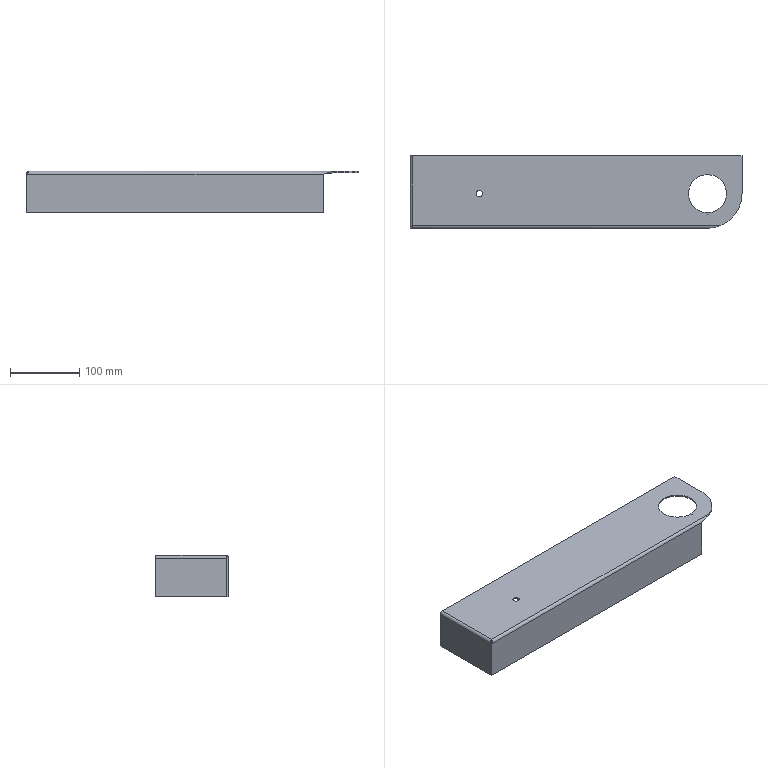Part | NX | features solid 2 | 1 solid | 34 faces | box 480 x 105 x 60 mm | volume 155228 mm3 | plane 22 | cylinder 8 | spline 4 | commonest cylinder face diameters 4 x2 8 x2 9 x2 55.2 x1 100 x1
STEP:
#1=CARTESIAN_POINT('',(-449.9,-1665.,358.));
#2=VERTEX_POINT('',#1);
#3=CARTESIAN_POINT('',(-449.9,-1662.6,358.));
#4=VERTEX_POINT('',#3);
#5=CARTESIAN_POINT('',(-449.9,-1685.,358.));
#6=DIRECTION('',(0.,1.,0.));
#7=VECTOR('',#6,1000.);
#8=LINE('',#5,#7);
#9=EDGE_CURVE('',#2,#4,#8,.T.);
#10=ORIENTED_EDGE('',*,*,#9,.F.);
#11=CARTESIAN_POINT('',(-449.9,-1665.,360.));
#12=VERTEX_POINT('',#11);
#13=CARTESIAN_POINT('',(-449.9,-1665.,360.));
#14=DIRECTION('',(0.,0.,1.));
#15=VECTOR('',#14,1000.);
#16=LINE('',#13,#15);
#17=EDGE_CURVE('',#2,#12,#16,.T.);
#18=ORIENTED_EDGE('',*,*,#17,.T.);
#19=CARTESIAN_POINT('',(-449.9,-1662.6,360.));
#20=VERTEX_POINT('',#19);
#21=CARTESIAN_POINT('',(-449.9,-1685.,360.));
#22=DIRECTION('',(0.,1.,0.));
#23=VECTOR('',#22,1000.);
#24=LINE('',#21,#23);
#25=EDGE_CURVE('',#12,#20,#24,.T.);
#26=ORIENTED_EDGE('',*,*,#25,.T.);
#27=CARTESIAN_POINT('',(-449.9,-1662.6,360.));
#28=DIRECTION('',(0.,0.,1.));
#29=VECTOR('',#28,1000.);
#30=LINE('',#27,#29);
#31=EDGE_CURVE('',#4,#20,#30,.T.);
#32=ORIENTED_EDGE('',*,*,#31,.F.);
#33=EDGE_LOOP('',(#10,#18,#26,#32));
#34=FACE_BOUND('',#33,.T.);
#35=CARTESIAN_POINT('',(-449.9,-1685.,360.));
#36=DIRECTION('',(1.,0.,0.));
#37=DIRECTION('',(0.,1.,0.));
#38=AXIS2_PLACEMENT_3D('',#35,#36,#37);
#39=PLANE('',#38);
#40=ADVANCED_FACE('',(#34),#39,.F.);
#41=CARTESIAN_POINT('',(-450.1,-1665.,358.));
#42=VERTEX_POINT('',#41);
#43=CARTESIAN_POINT('',(-450.1,-1665.,360.));
#44=VERTEX_POINT('',#43);
#45=CARTESIAN_POINT('',(-450.1,-1665.,360.));
#46=DIRECTION('',(0.,0.,1.));
#47=VECTOR('',#46,1000.);
#48=LINE('',#45,#47);
#49=EDGE_CURVE('',#42,#44,#48,.T.);
#50=ORIENTED_EDGE('',*,*,#49,.T.);
#51=CARTESIAN_POINT('',(-790.,-1665.,360.));
#52=DIRECTION('',(1.,0.,0.));
#53=VECTOR('',#52,1000.);
#54=LINE('',#51,#53);
#55=EDGE_CURVE('',#44,#12,#54,.T.);
#56=ORIENTED_EDGE('',*,*,#55,.T.);
#57=ORIENTED_EDGE('',*,*,#17,.F.);
#58=CARTESIAN_POINT('',(-790.,-1665.,358.));
#59=DIRECTION('',(1.,0.,0.));
#60=VECTOR('',#59,1000.);
#61=LINE('',#58,#60);
#62=EDGE_CURVE('',#42,#2,#61,.T.);
#63=ORIENTED_EDGE('',*,*,#62,.F.);
#64=EDGE_LOOP('',(#50,#56,#57,#63));
#65=FACE_BOUND('',#64,.T.);
#66=CARTESIAN_POINT('',(-790.,-1665.,360.));
#67=DIRECTION('',(0.,-1.,0.));
#68=DIRECTION('',(-1.,0.,0.));
#69=AXIS2_PLACEMENT_3D('',#66,#67,#68);
#70=PLANE('',#69);
#71=ADVANCED_FACE('',(#65),#70,.F.);
#72=CARTESIAN_POINT('',(-450.1,-1662.6,358.));
#73=VERTEX_POINT('',#72);
#74=CARTESIAN_POINT('',(-450.1,-1662.6,360.));
#75=VERTEX_POINT('',#74);
#76=CARTESIAN_POINT('',(-450.1,-1662.6,360.));
#77=DIRECTION('',(0.,0.,1.));
#78=VECTOR('',#77,1000.);
#79=LINE('',#76,#78);
#80=EDGE_CURVE('',#73,#75,#79,.T.);
#81=ORIENTED_EDGE('',*,*,#80,.T.);
#82=CARTESIAN_POINT('',(-450.1,-1685.,360.));
#83=DIRECTION('',(0.,-1.,0.));
#84=VECTOR('',#83,1000.);
#85=LINE('',#82,#84);
#86=EDGE_CURVE('',#75,#44,#85,.T.);
#87=ORIENTED_EDGE('',*,*,#86,.T.);
#88=ORIENTED_EDGE('',*,*,#49,.F.);
#89=CARTESIAN_POINT('',(-450.1,-1685.,358.));
#90=DIRECTION('',(0.,-1.,0.));
#91=VECTOR('',#90,1000.);
#92=LINE('',#89,#91);
#93=EDGE_CURVE('',#73,#42,#92,.T.);
#94=ORIENTED_EDGE('',*,*,#93,.F.);
#95=EDGE_LOOP('',(#81,#87,#88,#94));
#96=FACE_BOUND('',#95,.T.);
#97=CARTESIAN_POINT('',(-450.1,-1685.,360.));
#98=DIRECTION('',(-1.,0.,0.));
#99=DIRECTION('',(0.,1.,0.));
#100=AXIS2_PLACEMENT_3D('',#97,#98,#99);
#101=PLANE('',#100);
#102=ADVANCED_FACE('',(#96),#101,.F.);
#103=CARTESIAN_POINT('',(-780.,-1639.5,360.));
#104=VERTEX_POINT('',#103);
#105=CARTESIAN_POINT('',(-780.,-1639.5,358.));
#106=VERTEX_POINT('',#105);
#107=CARTESIAN_POINT('',(-780.,-1639.5,766.32));
#108=DIRECTION('',(0.,0.,-1.));
#109=VECTOR('',#108,1000.);
#110=LINE('',#107,#109);
#111=EDGE_CURVE('',#104,#106,#110,.T.);
#112=ORIENTED_EDGE('',*,*,#111,.F.);
#113=CARTESIAN_POINT('',(-780.,-1630.5,360.));
#114=VERTEX_POINT('',#113);
#115=CARTESIAN_POINT('',(-780.,-1635.,360.));
#116=DIRECTION('',(0.,0.,-1.));
#117=DIRECTION('',(0.,-1.,0.));
#118=AXIS2_PLACEMENT_3D('',#115,#116,#117);
#119=CIRCLE('',#118,4.5);
#120=EDGE_CURVE('',#114,#104,#119,.T.);
#121=ORIENTED_EDGE('',*,*,#120,.F.);
#122=CARTESIAN_POINT('',(-780.,-1630.5,358.));
#123=VERTEX_POINT('',#122);
#124=CARTESIAN_POINT('',(-780.,-1630.5,766.32));
#125=DIRECTION('',(0.,0.,-1.));
#126=VECTOR('',#125,1000.);
#127=LINE('',#124,#126);
#128=EDGE_CURVE('',#123,#114,#127,.F.);
#129=ORIENTED_EDGE('',*,*,#128,.F.);
#130=CARTESIAN_POINT('',(-780.,-1635.,358.));
#131=DIRECTION('',(0.,0.,1.));
#132=DIRECTION('',(-1.,0.,0.));
#133=AXIS2_PLACEMENT_3D('',#130,#131,#132);
#134=CIRCLE('',#133,4.5);
#135=EDGE_CURVE('',#106,#123,#134,.T.);
#136=ORIENTED_EDGE('',*,*,#135,.F.);
#137=EDGE_LOOP('',(#112,#121,#129,#136));
#138=FACE_BOUND('',#137,.T.);
#139=CARTESIAN_POINT('',(-780.,-1635.,766.32));
#140=DIRECTION('',(0.,0.,-1.));
#141=DIRECTION('',(0.,1.,0.));
#142=AXIS2_PLACEMENT_3D('',#139,#140,#141);
#143=CYLINDRICAL_SURFACE('',#142,4.5);
#144=ADVANCED_FACE('',(#138),#143,.F.);
#145=CARTESIAN_POINT('',(-450.,-1685.,356.));
#146=VERTEX_POINT('',#145);
#147=CARTESIAN_POINT('',(-450.,-1685.,300.));
#148=VERTEX_POINT('',#147);
#149=CARTESIAN_POINT('',(-450.,-1685.,-51.106));
#150=DIRECTION('',(0.,0.,-1.));
#151=VECTOR('',#150,1000.);
#152=LINE('',#149,#151);
#153=EDGE_CURVE('',#146,#148,#152,.T.);
#154=ORIENTED_EDGE('',*,*,#153,.F.);
#155=CARTESIAN_POINT('',(-877.9,-1685.,356.));
#156=VERTEX_POINT('',#155);
#157=CARTESIAN_POINT('',(-790.,-1685.,356.));
#158=DIRECTION('',(1.,0.,0.));
#159=VECTOR('',#158,1000.);
#160=LINE('',#157,#159);
#161=EDGE_CURVE('',#156,#146,#160,.T.);
#162=ORIENTED_EDGE('',*,*,#161,.F.);
#163=CARTESIAN_POINT('',(-880.,-1685.,356.));
#164=VERTEX_POINT('',#163);
#165=CARTESIAN_POINT('',(-880.,-1685.,356.));
#166=DIRECTION('',(1.,0.,0.));
#167=VECTOR('',#166,1000.);
#168=LINE('',#165,#167);
#169=EDGE_CURVE('',#164,#156,#168,.T.);
#170=ORIENTED_EDGE('',*,*,#169,.F.);
#171=CARTESIAN_POINT('',(-880.,-1685.,300.));
#172=VERTEX_POINT('',#171);
#173=CARTESIAN_POINT('',(-880.,-1685.,300.));
#174=DIRECTION('',(0.,0.,1.));
#175=VECTOR('',#174,1000.);
#176=LINE('',#173,#175);
#177=EDGE_CURVE('',#172,#164,#176,.T.);
#178=ORIENTED_EDGE('',*,*,#177,.F.);
#179=CARTESIAN_POINT('',(-790.,-1685.,300.));
#180=DIRECTION('',(1.,0.,0.));
#181=VECTOR('',#180,1000.);
#182=LINE('',#179,#181);
#183=EDGE_CURVE('',#172,#148,#182,.T.);
#184=ORIENTED_EDGE('',*,*,#183,.T.);
#185=EDGE_LOOP('',(#154,#162,#170,#178,#184));
#186=FACE_BOUND('',#185,.T.);
#187=CARTESIAN_POINT('',(-790.,-1685.,300.));
#188=DIRECTION('',(0.,-1.,0.));
#189=DIRECTION('',(-1.,0.,0.));
#190=AXIS2_PLACEMENT_3D('',#187,#188,#189);
#191=PLANE('',#190);
#192=ADVANCED_FACE('',(#186),#191,.T.);
#193=CARTESIAN_POINT('',(-880.,-1683.,356.));
#194=VERTEX_POINT('',#193);
#195=CARTESIAN_POINT('',(-880.,-1685.,356.));
#196=DIRECTION('',(0.,1.,0.));
#197=VECTOR('',#196,1000.);
#198=LINE('',#195,#197);
#199=EDGE_CURVE('',#164,#194,#198,.T.);
#200=ORIENTED_EDGE('',*,*,#199,.T.);
#201=CARTESIAN_POINT('',(-880.,-1683.,300.));
#202=VERTEX_POINT('',#201);
#203=CARTESIAN_POINT('',(-880.,-1683.,300.));
#204=DIRECTION('',(0.,0.,1.));
#205=VECTOR('',#204,1000.);
#206=LINE('',#203,#205);
#207=EDGE_CURVE('',#202,#194,#206,.T.);
#208=ORIENTED_EDGE('',*,*,#207,.F.);
#209=CARTESIAN_POINT('',(-880.,-1685.,300.));
#210=DIRECTION('',(0.,-1.,0.));
#211=VECTOR('',#210,1000.);
#212=LINE('',#209,#211);
#213=EDGE_CURVE('',#202,#172,#212,.T.);
#214=ORIENTED_EDGE('',*,*,#213,.T.);
#215=ORIENTED_EDGE('',*,*,#177,.T.);
#216=EDGE_LOOP('',(#200,#208,#214,#215));
#217=FACE_BOUND('',#216,.T.);
#218=CARTESIAN_POINT('',(-880.,-1685.,360.));
#219=DIRECTION('',(-1.,0.,0.));
#220=DIRECTION('',(0.,1.,0.));
#221=AXIS2_PLACEMENT_3D('',#218,#219,#220);
#222=PLANE('',#221);
#223=ADVANCED_FACE('',(#217),#222,.T.);
#224=CARTESIAN_POINT('',(-450.,-1683.,300.));
#225=VERTEX_POINT('',#224);
#226=CARTESIAN_POINT('',(-790.,-1683.,300.));
#227=DIRECTION('',(1.,0.,0.));
#228=VECTOR('',#227,1000.);
#229=LINE('',#226,#228);
#230=EDGE_CURVE('',#202,#225,#229,.T.);
#231=ORIENTED_EDGE('',*,*,#230,.F.);
#232=ORIENTED_EDGE('',*,*,#207,.T.);
#233=CARTESIAN_POINT('',(-877.9,-1683.,356.));
#234=VERTEX_POINT('',#233);
#235=CARTESIAN_POINT('',(-880.,-1683.,356.));
#236=DIRECTION('',(1.,0.,0.));
#237=VECTOR('',#236,1000.);
#238=LINE('',#235,#237);
#239=EDGE_CURVE('',#194,#234,#238,.T.);
#240=ORIENTED_EDGE('',*,*,#239,.T.);
#241=CARTESIAN_POINT('',(-450.,-1683.,356.));
#242=VERTEX_POINT('',#241);
#243=CARTESIAN_POINT('',(-790.,-1683.,356.));
#244=DIRECTION('',(1.,0.,0.));
#245=VECTOR('',#244,1000.);
#246=LINE('',#243,#245);
#247=EDGE_CURVE('',#234,#242,#246,.T.);
#248=ORIENTED_EDGE('',*,*,#247,.T.);
#249=CARTESIAN_POINT('',(-450.,-1683.,300.));
#250=DIRECTION('',(0.,0.,-1.));
#251=VECTOR('',#250,1000.);
#252=LINE('',#249,#251);
#253=EDGE_CURVE('',#242,#225,#252,.T.);
#254=ORIENTED_EDGE('',*,*,#253,.T.);
#255=EDGE_LOOP('',(#231,#232,#240,#248,#254));
#256=FACE_BOUND('',#255,.T.);
#257=CARTESIAN_POINT('',(-790.,-1683.,300.));
#258=DIRECTION('',(0.,-1.,0.));
#259=DIRECTION('',(-1.,0.,0.));
#260=AXIS2_PLACEMENT_3D('',#257,#258,#259);
#261=PLANE('',#260);
#262=ADVANCED_FACE('',(#256),#261,.F.);
#263=CARTESIAN_POINT('',(-450.,-1685.,300.));
#264=DIRECTION('',(0.,-1.,0.));
#265=VECTOR('',#264,1000.);
#266=LINE('',#263,#265);
#267=EDGE_CURVE('',#225,#148,#266,.T.);
#268=ORIENTED_EDGE('',*,*,#267,.F.);
#269=ORIENTED_EDGE('',*,*,#253,.F.);
#270=CARTESIAN_POINT('',(-450.,-1685.,356.));
#271=DIRECTION('',(0.,-1.,0.));
#272=VECTOR('',#271,1000.);
#273=LINE('',#270,#272);
#274=EDGE_CURVE('',#242,#146,#273,.T.);
#275=ORIENTED_EDGE('',*,*,#274,.T.);
#276=ORIENTED_EDGE('',*,*,#153,.T.);
#277=EDGE_LOOP('',(#268,#269,#275,#276));
#278=FACE_BOUND('',#277,.T.);
#279=CARTESIAN_POINT('',(-450.,-1685.,-51.106));
#280=DIRECTION('',(-1.,0.,0.));
#281=DIRECTION('',(0.,1.,0.));
#282=AXIS2_PLACEMENT_3D('',#279,#280,#281);
#283=PLANE('',#282);
#284=ADVANCED_FACE('',(#278),#283,.F.);
#285=ORIENTED_EDGE('',*,*,#267,.T.);
#286=ORIENTED_EDGE('',*,*,#183,.F.);
#287=ORIENTED_EDGE('',*,*,#213,.F.);
#288=ORIENTED_EDGE('',*,*,#230,.T.);
#289=EDGE_LOOP('',(#285,#286,#287,#288));
#290=FACE_BOUND('',#289,.T.);
#291=CARTESIAN_POINT('',(-790.,-1685.,300.));
#292=DIRECTION('',(0.,0.,1.));
#293=DIRECTION('',(0.,-1.,0.));
#294=AXIS2_PLACEMENT_3D('',#291,#292,#293);
#295=PLANE('',#294);
#296=ADVANCED_FACE('',(#290),#295,.F.);
#297=CARTESIAN_POINT('',(-877.9,-1683.,356.));
#298=DIRECTION('',(0.,1.,0.));
#299=VECTOR('',#298,1000.);
#300=LINE('',#297,#299);
#301=EDGE_CURVE('',#156,#234,#300,.T.);
#302=ORIENTED_EDGE('',*,*,#301,.T.);
#303=ORIENTED_EDGE('',*,*,#239,.F.);
#304=ORIENTED_EDGE('',*,*,#199,.F.);
#305=ORIENTED_EDGE('',*,*,#169,.T.);
#306=EDGE_LOOP('',(#302,#303,#304,#305));
#307=FACE_BOUND('',#306,.T.);
#308=CARTESIAN_POINT('',(-540.,-1685.,356.));
#309=DIRECTION('',(0.,0.,-1.));
#310=DIRECTION('',(0.,-1.,0.));
#311=AXIS2_PLACEMENT_3D('',#308,#309,#310);
#312=PLANE('',#311);
#313=ADVANCED_FACE('',(#307),#312,.F.);
#314=CARTESIAN_POINT('',(-876.977,-1682.028,357.716));
#315=VERTEX_POINT('',#314);
#316=CARTESIAN_POINT('',(-877.396,-1682.469,359.72));
#317=VERTEX_POINT('',#316);
#318=CARTESIAN_POINT('',(-876.977,-1682.028,357.716));
#319=CARTESIAN_POINT('',(-877.12,-1682.179,358.298));
#320=CARTESIAN_POINT('',(-877.26,-1682.326,358.966));
#321=CARTESIAN_POINT('',(-877.396,-1682.469,359.72));
#322=B_SPLINE_CURVE_WITH_KNOTS('',3,(#318,#319,#320,#321),.UNSPECIFIED.,.F.,.F.,(4,4),(0.,1.),.UNSPECIFIED.);
#323=EDGE_CURVE('',#315,#317,#322,.T.);
#324=ORIENTED_EDGE('',*,*,#323,.F.);
#325=CARTESIAN_POINT('',(-877.817,-1682.913,356.584));
#326=VERTEX_POINT('',#325);
#327=CARTESIAN_POINT('',(-877.817,-1682.913,356.584));
#328=CARTESIAN_POINT('',(-877.411,-1682.884,356.68));
#329=CARTESIAN_POINT('',(-876.704,-1682.733,357.125));
#330=CARTESIAN_POINT('',(-876.747,-1682.261,357.576));
#331=CARTESIAN_POINT('',(-876.977,-1682.028,357.716));
#332=B_SPLINE_CURVE_WITH_KNOTS('',3,(#327,#328,#329,#330,#331),.UNSPECIFIED.,.F.,.F.,(4,1,4),(0.,0.5,1.),.UNSPECIFIED.);
#333=EDGE_CURVE('',#315,#326,#332,.F.);
#334=ORIENTED_EDGE('',*,*,#333,.T.);
#335=CARTESIAN_POINT('',(-877.9,-1683.,356.59));
#336=VERTEX_POINT('',#335);
#337=CARTESIAN_POINT('',(-877.9,-1683.,356.59));
#338=CARTESIAN_POINT('',(-877.872,-1682.971,356.588));
#339=CARTESIAN_POINT('',(-877.845,-1682.942,356.586));
#340=CARTESIAN_POINT('',(-877.817,-1682.913,356.584));
#341=(BOUNDED_CURVE()B_SPLINE_CURVE(3,(#337,#338,#339,#340),.UNSPECIFIED.,.F.,.F.)B_SPLINE_CURVE_WITH_KNOTS((4,4),(0.,0.0001204),.PIECEWISE_BEZIER_KNOTS.)CURVE()GEOMETRIC_REPRESENTATION_ITEM()RATIONAL_B_SPLINE_CURVE((1.,1.,1.,1.))REPRESENTATION_ITEM(''));
#342=EDGE_CURVE('',#336,#326,#341,.T.);
#343=ORIENTED_EDGE('',*,*,#342,.F.);
#344=CARTESIAN_POINT('',(-877.9,-1684.836,357.132));
#345=VERTEX_POINT('',#344);
#346=CARTESIAN_POINT('',(-877.9,-1684.836,357.132));
#347=CARTESIAN_POINT('',(-877.9,-1684.224,356.952));
#348=CARTESIAN_POINT('',(-877.9,-1683.612,356.771));
#349=CARTESIAN_POINT('',(-877.9,-1683.,356.59));
#350=(BOUNDED_CURVE()B_SPLINE_CURVE(3,(#346,#347,#348,#349),.UNSPECIFIED.,.F.,.F.)B_SPLINE_CURVE_WITH_KNOTS((4,4),(0.000001137,0.001916),.PIECEWISE_BEZIER_KNOTS.)CURVE()GEOMETRIC_REPRESENTATION_ITEM()RATIONAL_B_SPLINE_CURVE((1.,1.,1.,1.))REPRESENTATION_ITEM(''));
#351=EDGE_CURVE('',#345,#336,#350,.T.);
#352=ORIENTED_EDGE('',*,*,#351,.F.);
#353=CARTESIAN_POINT('',(-877.396,-1682.469,359.72));
#354=CARTESIAN_POINT('',(-876.928,-1682.929,359.539));
#355=CARTESIAN_POINT('',(-876.617,-1683.907,358.913));
#356=CARTESIAN_POINT('',(-877.053,-1684.627,357.77));
#357=CARTESIAN_POINT('',(-877.601,-1684.802,357.248));
#358=CARTESIAN_POINT('',(-877.9,-1684.836,357.132));
#359=B_SPLINE_CURVE_WITH_KNOTS('',3,(#353,#354,#355,#356,#357,#358),.UNSPECIFIED.,.F.,.F.,(4,1,1,4),(0.,0.5,0.75,1.),.UNSPECIFIED.);
#360=EDGE_CURVE('',#317,#345,#359,.T.);
#361=ORIENTED_EDGE('',*,*,#360,.F.);
#362=EDGE_LOOP('',(#324,#334,#343,#352,#361));
#363=FACE_BOUND('',#362,.T.);
#364=CARTESIAN_POINT('',(-878.278,-1684.858,357.06));
#365=CARTESIAN_POINT('',(-878.474,-1684.858,357.06));
#366=CARTESIAN_POINT('',(-878.666,-1684.843,357.12));
#367=CARTESIAN_POINT('',(-879.021,-1684.776,357.328));
#368=CARTESIAN_POINT('',(-879.184,-1684.723,357.477));
#369=CARTESIAN_POINT('',(-879.461,-1684.566,357.824));
#370=CARTESIAN_POINT('',(-879.574,-1684.46,358.024));
#371=CARTESIAN_POINT('',(-879.733,-1684.188,358.43));
#372=CARTESIAN_POINT('',(-879.778,-1684.021,358.638));
#373=CARTESIAN_POINT('',(-879.778,-1683.638,359.021));
#374=CARTESIAN_POINT('',(-879.733,-1683.43,359.188));
#375=CARTESIAN_POINT('',(-879.574,-1683.024,359.46));
#376=CARTESIAN_POINT('',(-879.461,-1682.824,359.566));
#377=CARTESIAN_POINT('',(-879.184,-1682.477,359.723));
#378=CARTESIAN_POINT('',(-879.021,-1682.328,359.776));
#379=CARTESIAN_POINT('',(-878.666,-1682.12,359.843));
#380=CARTESIAN_POINT('',(-878.474,-1682.06,359.858));
#381=CARTESIAN_POINT('',(-878.081,-1682.06,359.858));
#382=CARTESIAN_POINT('',(-877.889,-1682.12,359.843));
#383=CARTESIAN_POINT('',(-877.534,-1682.328,359.776));
#384=CARTESIAN_POINT('',(-877.372,-1682.477,359.723));
#385=CARTESIAN_POINT('',(-877.095,-1682.824,359.566));
#386=CARTESIAN_POINT('',(-876.981,-1683.024,359.46));
#387=CARTESIAN_POINT('',(-876.822,-1683.43,359.188));
#388=CARTESIAN_POINT('',(-876.778,-1683.638,359.021));
#389=CARTESIAN_POINT('',(-876.778,-1684.021,358.638));
#390=CARTESIAN_POINT('',(-876.822,-1684.188,358.43));
#391=CARTESIAN_POINT('',(-876.981,-1684.46,358.024));
#392=CARTESIAN_POINT('',(-877.095,-1684.566,357.824));
#393=CARTESIAN_POINT('',(-877.372,-1684.723,357.477));
#394=CARTESIAN_POINT('',(-877.534,-1684.776,357.328));
#395=CARTESIAN_POINT('',(-877.889,-1684.843,357.12));
#396=CARTESIAN_POINT('',(-878.081,-1684.858,357.06));
#397=CARTESIAN_POINT('',(-878.278,-1684.858,357.06));
#398=CARTESIAN_POINT('',(-878.278,-1682.928,356.53));
#399=CARTESIAN_POINT('',(-878.474,-1682.928,356.53));
#400=CARTESIAN_POINT('',(-878.666,-1682.92,356.559));
#401=CARTESIAN_POINT('',(-879.021,-1682.886,356.664));
#402=CARTESIAN_POINT('',(-879.184,-1682.86,356.738));
#403=CARTESIAN_POINT('',(-879.461,-1682.782,356.912));
#404=CARTESIAN_POINT('',(-879.574,-1682.729,357.011));
#405=CARTESIAN_POINT('',(-879.733,-1682.593,357.214));
#406=CARTESIAN_POINT('',(-879.778,-1682.509,357.318));
#407=CARTESIAN_POINT('',(-879.778,-1682.318,357.509));
#408=CARTESIAN_POINT('',(-879.733,-1682.214,357.593));
#409=CARTESIAN_POINT('',(-879.574,-1682.011,357.729));
#410=CARTESIAN_POINT('',(-879.461,-1681.912,357.782));
#411=CARTESIAN_POINT('',(-879.184,-1681.738,357.86));
#412=CARTESIAN_POINT('',(-879.021,-1681.664,357.886));
#413=CARTESIAN_POINT('',(-878.666,-1681.559,357.92));
#414=CARTESIAN_POINT('',(-878.474,-1681.53,357.928));
#415=CARTESIAN_POINT('',(-878.081,-1681.53,357.928));
#416=CARTESIAN_POINT('',(-877.889,-1681.559,357.92));
#417=CARTESIAN_POINT('',(-877.534,-1681.664,357.886));
#418=CARTESIAN_POINT('',(-877.372,-1681.738,357.86));
#419=CARTESIAN_POINT('',(-877.095,-1681.912,357.782));
#420=CARTESIAN_POINT('',(-876.981,-1682.011,357.729));
#421=CARTESIAN_POINT('',(-876.822,-1682.214,357.593));
#422=CARTESIAN_POINT('',(-876.778,-1682.318,357.509));
#423=CARTESIAN_POINT('',(-876.778,-1682.509,357.318));
#424=CARTESIAN_POINT('',(-876.822,-1682.593,357.214));
#425=CARTESIAN_POINT('',(-876.981,-1682.729,357.011));
#426=CARTESIAN_POINT('',(-877.095,-1682.782,356.912));
#427=CARTESIAN_POINT('',(-877.372,-1682.86,356.738));
#428=CARTESIAN_POINT('',(-877.534,-1682.886,356.664));
#429=CARTESIAN_POINT('',(-877.889,-1682.92,356.559));
#430=CARTESIAN_POINT('',(-878.081,-1682.928,356.53));
#431=CARTESIAN_POINT('',(-878.278,-1682.928,356.53));
#432=(BOUNDED_SURFACE()B_SPLINE_SURFACE(1,3,((#364,#365,#366,#367,#368,#369,#370,#371,#372,#373,#374,#375,#376,#377,#378,#379,#380,#381,#382,#383,#384,#385,#386,#387,#388,#389,#390,#391,#392,#393,#394,#395,#396,#397),(#398,#399,#400,#401,#402,#403,#404,#405,#406,#407,#408,#409,#410,#411,#412,#413,#414,#415,#416,#417,#418,#419,#420,#421,#422,#423,#424,#425,#426,#427,#428,#429,#430,#431)),.RULED_SURF.,.F.,.T.,.F.)B_SPLINE_SURFACE_WITH_KNOTS((2,2),(1,3,2,2,2,2,2,2,2,2,2,2,2,2,2,2,2,3,1),(0.,1.),(-0.3927,0.,0.3927,0.7854,1.178,1.571,1.963,2.356,2.749,3.142,3.534,3.927,4.32,4.712,5.105,5.498,5.89,6.283,6.676),.UNSPECIFIED.)GEOMETRIC_REPRESENTATION_ITEM()RATIONAL_B_SPLINE_SURFACE(((1.,1.,1.,1.,1.,1.,1.,1.,1.,1.,1.,1.,1.,1.,1.,1.,1.,1.,1.,1.,1.,1.,1.,1.,1.,1.,1.,1.,1.,1.,1.,1.,1.,1.),(1.,1.,1.,1.,1.,1.,1.,1.,1.,1.,1.,1.,1.,1.,1.,1.,1.,1.,1.,1.,1.,1.,1.,1.,1.,1.,1.,1.,1.,1.,1.,1.,1.,1.)))REPRESENTATION_ITEM('')SURFACE());
#433=ADVANCED_FACE('',(#363),#432,.T.);
#434=ORIENTED_EDGE('',*,*,#351,.T.);
#435=CARTESIAN_POINT('',(-877.9,-1683.,-640.));
#436=DIRECTION('',(0.,0.,-1.));
#437=VECTOR('',#436,1000.);
#438=LINE('',#435,#437);
#439=EDGE_CURVE('',#336,#234,#438,.T.);
#440=ORIENTED_EDGE('',*,*,#439,.T.);
#441=ORIENTED_EDGE('',*,*,#301,.F.);
#442=CARTESIAN_POINT('',(-877.9,-1681.,356.));
#443=DIRECTION('',(-1.,0.,0.));
#444=DIRECTION('',(0.,0.,1.));
#445=AXIS2_PLACEMENT_3D('',#442,#443,#444);
#446=CIRCLE('',#445,4.);
#447=EDGE_CURVE('',#156,#345,#446,.T.);
#448=ORIENTED_EDGE('',*,*,#447,.T.);
#449=EDGE_LOOP('',(#434,#440,#441,#448));
#450=FACE_BOUND('',#449,.T.);
#451=CARTESIAN_POINT('',(-877.9,-1683.,1360.));
#452=DIRECTION('',(-1.,0.,0.));
#453=DIRECTION('',(0.,1.,0.));
#454=AXIS2_PLACEMENT_3D('',#451,#452,#453);
#455=PLANE('',#454);
#456=ADVANCED_FACE('',(#450),#455,.T.);
#457=ORIENTED_EDGE('',*,*,#323,.T.);
#458=CARTESIAN_POINT('',(-876.,-1681.,360.));
#459=VERTEX_POINT('',#458);
#460=CARTESIAN_POINT('',(-877.396,-1682.469,359.72));
#461=CARTESIAN_POINT('',(-876.95,-1682.,359.906));
#462=CARTESIAN_POINT('',(-876.479,-1681.504,360.));
#463=CARTESIAN_POINT('',(-876.,-1681.,360.));
#464=(BOUNDED_CURVE()B_SPLINE_CURVE(3,(#460,#461,#462,#463),.UNSPECIFIED.,.F.,.F.)B_SPLINE_CURVE_WITH_KNOTS((4,4),(4.336,4.712),.PIECEWISE_BEZIER_KNOTS.)CURVE()GEOMETRIC_REPRESENTATION_ITEM()RATIONAL_B_SPLINE_CURVE((1.,0.9882,0.9882,1.))REPRESENTATION_ITEM(''));
#465=EDGE_CURVE('',#317,#459,#464,.T.);
#466=ORIENTED_EDGE('',*,*,#465,.T.);
#467=CARTESIAN_POINT('',(-876.,-1681.,358.));
#468=VERTEX_POINT('',#467);
#469=CARTESIAN_POINT('',(-876.,-1681.,360.));
#470=DIRECTION('',(0.,0.,1.));
#471=VECTOR('',#470,1000.);
#472=LINE('',#469,#471);
#473=EDGE_CURVE('',#468,#459,#472,.T.);
#474=ORIENTED_EDGE('',*,*,#473,.F.);
#475=CARTESIAN_POINT('',(-876.977,-1682.028,357.716));
#476=CARTESIAN_POINT('',(-876.68,-1681.716,357.903));
#477=CARTESIAN_POINT('',(-876.346,-1681.364,358.));
#478=CARTESIAN_POINT('',(-876.,-1681.,358.));
#479=(BOUNDED_CURVE()B_SPLINE_CURVE(3,(#475,#476,#477,#478),.UNSPECIFIED.,.F.,.F.)B_SPLINE_CURVE_WITH_KNOTS((4,4),(4.173,4.712),.PIECEWISE_BEZIER_KNOTS.)CURVE()GEOMETRIC_REPRESENTATION_ITEM()RATIONAL_B_SPLINE_CURVE((1.,0.9759,0.9759,1.))REPRESENTATION_ITEM(''));
#480=EDGE_CURVE('',#315,#468,#479,.T.);
#481=ORIENTED_EDGE('',*,*,#480,.F.);
#482=EDGE_LOOP('',(#457,#466,#474,#481));
#483=FACE_BOUND('',#482,.T.);
#484=CARTESIAN_POINT('',(-187.251,-956.001,1360.));
#485=DIRECTION('',(-0.725,0.6887,0.));
#486=DIRECTION('',(0.,0.,1.));
#487=AXIS2_PLACEMENT_3D('',#484,#485,#486);
#488=PLANE('',#487);
#489=ADVANCED_FACE('',(#483),#488,.T.);
#490=CARTESIAN_POINT('',(-440.695,-1682.563,357.247));
#491=VERTEX_POINT('',#490);
#492=CARTESIAN_POINT('',(-440.695,-1684.127,358.495));
#493=VERTEX_POINT('',#492);
#494=CARTESIAN_POINT('',(-440.695,-1683.345,357.871));
#495=DIRECTION('',(0.,-0.7816,0.6237));
#496=VECTOR('',#495,1000.);
#497=LINE('',#494,#496);
#498=EDGE_CURVE('',#491,#493,#497,.T.);
#499=ORIENTED_EDGE('',*,*,#498,.F.);
#500=CARTESIAN_POINT('',(-430.404,-1681.,358.));
#501=VERTEX_POINT('',#500);
#502=CARTESIAN_POINT('',(-430.404,-1681.,358.));
#503=CARTESIAN_POINT('',(-431.126,-1681.154,358.));
#504=CARTESIAN_POINT('',(-432.3,-1681.389,357.974));
#505=CARTESIAN_POINT('',(-433.859,-1681.663,357.89));
#506=CARTESIAN_POINT('',(-434.771,-1681.813,357.829));
#507=CARTESIAN_POINT('',(-435.556,-1681.935,357.769));
#508=CARTESIAN_POINT('',(-436.071,-1682.011,357.727));
#509=CARTESIAN_POINT('',(-436.886,-1682.126,357.655));
#510=CARTESIAN_POINT('',(-438.337,-1682.317,357.516));
#511=CARTESIAN_POINT('',(-439.721,-1682.471,357.363));
#512=CARTESIAN_POINT('',(-440.695,-1682.563,357.247));
#513=B_SPLINE_CURVE_WITH_KNOTS('',3,(#502,#503,#504,#505,#506,#507,#508,#509,#510,#511,#512),.UNSPECIFIED.,.F.,.F.,(4,1,1,1,1,1,1,1,4),(0.,0.25,0.375,0.4375,0.5,0.5625,0.625,0.75,1.),.UNSPECIFIED.);
#514=EDGE_CURVE('',#491,#501,#513,.F.);
#515=ORIENTED_EDGE('',*,*,#514,.T.);
#516=CARTESIAN_POINT('',(-430.404,-1681.,360.));
#517=VERTEX_POINT('',#516);
#518=CARTESIAN_POINT('',(-430.404,-1681.,360.));
#519=DIRECTION('',(0.,0.,1.));
#520=VECTOR('',#519,1000.);
#521=LINE('',#518,#520);
#522=EDGE_CURVE('',#501,#517,#521,.T.);
#523=ORIENTED_EDGE('',*,*,#522,.T.);
#524=CARTESIAN_POINT('',(-440.695,-1684.127,358.495));
#525=CARTESIAN_POINT('',(-436.364,-1683.306,359.523));
#526=CARTESIAN_POINT('',(-432.933,-1682.077,360.));
#527=CARTESIAN_POINT('',(-430.404,-1681.,360.));
#528=B_SPLINE_CURVE_WITH_KNOTS('',3,(#524,#525,#526,#527),.UNSPECIFIED.,.F.,.F.,(4,4),(0.,1.),.UNSPECIFIED.);
#529=EDGE_CURVE('',#493,#517,#528,.T.);
#530=ORIENTED_EDGE('',*,*,#529,.F.);
#531=EDGE_LOOP('',(#499,#515,#523,#530));
#532=FACE_BOUND('',#531,.T.);
#533=CARTESIAN_POINT('',(-440.695,-1684.127,358.495));
#534=CARTESIAN_POINT('',(-438.952,-1683.796,358.909));
#535=CARTESIAN_POINT('',(-435.504,-1682.953,359.635));
#536=CARTESIAN_POINT('',(-432.083,-1681.716,359.997));
#537=CARTESIAN_POINT('',(-430.404,-1681.,360.));
#538=CARTESIAN_POINT('',(-440.695,-1683.605,358.079));
#539=CARTESIAN_POINT('',(-438.952,-1683.33,358.424));
#540=CARTESIAN_POINT('',(-435.504,-1682.628,359.03));
#541=CARTESIAN_POINT('',(-432.083,-1681.596,359.331));
#542=CARTESIAN_POINT('',(-430.404,-1681.,359.333));
#543=CARTESIAN_POINT('',(-440.695,-1683.084,357.663));
#544=CARTESIAN_POINT('',(-438.952,-1682.864,357.939));
#545=CARTESIAN_POINT('',(-435.504,-1682.302,358.424));
#546=CARTESIAN_POINT('',(-432.083,-1681.477,358.664));
#547=CARTESIAN_POINT('',(-430.404,-1681.,358.667));
#548=CARTESIAN_POINT('',(-440.695,-1682.563,357.247));
#549=CARTESIAN_POINT('',(-438.952,-1682.398,357.454));
#550=CARTESIAN_POINT('',(-435.504,-1681.977,357.818));
#551=CARTESIAN_POINT('',(-432.083,-1681.358,357.998));
#552=CARTESIAN_POINT('',(-430.404,-1681.,358.));
#553=(BOUNDED_SURFACE()B_SPLINE_SURFACE(3,3,((#533,#534,#535,#536,#537),(#538,#539,#540,#541,#542),(#543,#544,#545,#546,#547),(#548,#549,#550,#551,#552)),.UNSPECIFIED.,.F.,.F.,.F.)B_SPLINE_SURFACE_WITH_KNOTS((4,4),(4,1,4),(0.,1.),(0.,0.005437,0.01087),.UNSPECIFIED.)GEOMETRIC_REPRESENTATION_ITEM()RATIONAL_B_SPLINE_SURFACE(((1.,1.,1.,1.,1.),(1.,1.,1.,1.,1.),(1.,1.,1.,1.,1.),(1.,1.,1.,1.,1.)))REPRESENTATION_ITEM('')SURFACE());
#554=ADVANCED_FACE('',(#532),#553,.T.);
#555=ORIENTED_EDGE('',*,*,#274,.F.);
#556=CARTESIAN_POINT('',(-440.695,-1682.563,357.247));
#557=CARTESIAN_POINT('',(-441.363,-1682.627,357.168));
#558=CARTESIAN_POINT('',(-442.436,-1682.718,357.036));
#559=CARTESIAN_POINT('',(-443.857,-1682.812,356.85));
#560=CARTESIAN_POINT('',(-444.665,-1682.858,356.742));
#561=CARTESIAN_POINT('',(-445.415,-1682.895,356.641));
#562=CARTESIAN_POINT('',(-445.71,-1682.908,356.6));
#563=CARTESIAN_POINT('',(-446.349,-1682.934,356.513));
#564=CARTESIAN_POINT('',(-447.566,-1682.975,356.344));
#565=CARTESIAN_POINT('',(-448.947,-1683.,356.149));
#566=CARTESIAN_POINT('',(-450.,-1683.,356.));
#567=B_SPLINE_CURVE_WITH_KNOTS('',3,(#556,#557,#558,#559,#560,#561,#562,#563,#564,#565,#566),.UNSPECIFIED.,.F.,.F.,(4,1,1,1,1,1,1,1,4),(0.,0.25,0.375,0.4375,0.5,0.5625,0.625,0.75,1.),.UNSPECIFIED.);
#568=EDGE_CURVE('',#242,#491,#567,.F.);
#569=ORIENTED_EDGE('',*,*,#568,.T.);
#570=ORIENTED_EDGE('',*,*,#498,.T.);
#571=CARTESIAN_POINT('',(-450.,-1685.,356.));
#572=CARTESIAN_POINT('',(-449.01,-1685.,356.28));
#573=CARTESIAN_POINT('',(-447.677,-1684.956,356.657));
#574=CARTESIAN_POINT('',(-446.431,-1684.874,357.003));
#575=CARTESIAN_POINT('',(-445.758,-1684.82,357.188));
#576=CARTESIAN_POINT('',(-445.407,-1684.789,357.284));
#577=CARTESIAN_POINT('',(-444.66,-1684.716,357.486));
#578=CARTESIAN_POINT('',(-443.84,-1684.622,357.705));
#579=CARTESIAN_POINT('',(-442.415,-1684.433,358.077));
#580=CARTESIAN_POINT('',(-441.351,-1684.251,358.339));
#581=CARTESIAN_POINT('',(-440.695,-1684.127,358.495));
#582=B_SPLINE_CURVE_WITH_KNOTS('',3,(#571,#572,#573,#574,#575,#576,#577,#578,#579,#580,#581),.UNSPECIFIED.,.F.,.F.,(4,1,1,1,1,1,1,1,4),(0.,0.25,0.375,0.4375,0.5,0.5625,0.625,0.75,1.),.UNSPECIFIED.);
#583=EDGE_CURVE('',#146,#493,#582,.T.);
#584=ORIENTED_EDGE('',*,*,#583,.F.);
#585=EDGE_LOOP('',(#555,#569,#570,#584));
#586=FACE_BOUND('',#585,.T.);
#587=CARTESIAN_POINT('',(-440.695,-1684.127,358.495));
#588=CARTESIAN_POINT('',(-442.243,-1684.42,358.127));
#589=CARTESIAN_POINT('',(-445.335,-1684.855,357.319));
#590=CARTESIAN_POINT('',(-448.443,-1685.,356.44));
#591=CARTESIAN_POINT('',(-450.,-1685.,356.));
#592=CARTESIAN_POINT('',(-440.695,-1683.605,358.079));
#593=CARTESIAN_POINT('',(-442.243,-1683.85,357.773));
#594=CARTESIAN_POINT('',(-445.335,-1684.212,357.099));
#595=CARTESIAN_POINT('',(-448.443,-1684.333,356.367));
#596=CARTESIAN_POINT('',(-450.,-1684.333,356.));
#597=CARTESIAN_POINT('',(-440.695,-1683.084,357.663));
#598=CARTESIAN_POINT('',(-442.243,-1683.28,357.418));
#599=CARTESIAN_POINT('',(-445.335,-1683.57,356.88));
#600=CARTESIAN_POINT('',(-448.443,-1683.667,356.294));
#601=CARTESIAN_POINT('',(-450.,-1683.667,356.));
#602=CARTESIAN_POINT('',(-440.695,-1682.563,357.247));
#603=CARTESIAN_POINT('',(-442.243,-1682.71,357.064));
#604=CARTESIAN_POINT('',(-445.335,-1682.927,356.66));
#605=CARTESIAN_POINT('',(-448.443,-1683.,356.22));
#606=CARTESIAN_POINT('',(-450.,-1683.,356.));
#607=(BOUNDED_SURFACE()B_SPLINE_SURFACE(3,3,((#587,#588,#589,#590,#591),(#592,#593,#594,#595,#596),(#597,#598,#599,#600,#601),(#602,#603,#604,#605,#606)),.RULED_SURF.,.F.,.F.,.F.)B_SPLINE_SURFACE_WITH_KNOTS((4,4),(4,1,4),(0.,1.),(0.,0.004837,0.009674),.UNSPECIFIED.)GEOMETRIC_REPRESENTATION_ITEM()RATIONAL_B_SPLINE_SURFACE(((1.,1.,1.,1.,1.),(1.,1.,1.,1.,1.),(1.,1.,1.,1.,1.),(1.,1.,1.,1.,1.)))REPRESENTATION_ITEM('')SURFACE());
#608=ADVANCED_FACE('',(#586),#607,.F.);
#609=ORIENTED_EDGE('',*,*,#480,.T.);
#610=CARTESIAN_POINT('',(-790.,-1681.,358.));
#611=DIRECTION('',(1.,0.,0.));
#612=VECTOR('',#611,1000.);
#613=LINE('',#610,#612);
#614=EDGE_CURVE('',#468,#501,#613,.T.);
#615=ORIENTED_EDGE('',*,*,#614,.T.);
#616=ORIENTED_EDGE('',*,*,#514,.F.);
#617=ORIENTED_EDGE('',*,*,#568,.F.);
#618=ORIENTED_EDGE('',*,*,#247,.F.);
#619=CARTESIAN_POINT('',(-877.9,-1683.,356.));
#620=CARTESIAN_POINT('',(-877.9,-1683.,356.198));
#621=CARTESIAN_POINT('',(-877.872,-1682.971,356.394));
#622=CARTESIAN_POINT('',(-877.817,-1682.913,356.584));
#623=(BOUNDED_CURVE()B_SPLINE_CURVE(3,(#619,#620,#621,#622),.UNSPECIFIED.,.F.,.F.)B_SPLINE_CURVE_WITH_KNOTS((4,4),(3.142,3.438),.PIECEWISE_BEZIER_KNOTS.)CURVE()GEOMETRIC_REPRESENTATION_ITEM()RATIONAL_B_SPLINE_CURVE((1.,0.9927,0.9927,1.))REPRESENTATION_ITEM(''));
#624=EDGE_CURVE('',#234,#326,#623,.T.);
#625=ORIENTED_EDGE('',*,*,#624,.T.);
#626=ORIENTED_EDGE('',*,*,#333,.F.);
#627=EDGE_LOOP('',(#609,#615,#616,#617,#618,#625,#626));
#628=FACE_BOUND('',#627,.T.);
#629=CARTESIAN_POINT('',(-790.,-1681.,356.));
#630=DIRECTION('',(1.,0.,0.));
#631=DIRECTION('',(0.,0.,-1.));
#632=AXIS2_PLACEMENT_3D('',#629,#630,#631);
#633=CYLINDRICAL_SURFACE('',#632,2.);
#634=ADVANCED_FACE('',(#628),#633,.F.);
#635=ORIENTED_EDGE('',*,*,#360,.T.);
#636=ORIENTED_EDGE('',*,*,#447,.F.);
#637=ORIENTED_EDGE('',*,*,#161,.T.);
#638=ORIENTED_EDGE('',*,*,#583,.T.);
#639=ORIENTED_EDGE('',*,*,#529,.T.);
#640=CARTESIAN_POINT('',(-790.,-1681.,360.));
#641=DIRECTION('',(1.,0.,0.));
#642=VECTOR('',#641,1000.);
#643=LINE('',#640,#642);
#644=EDGE_CURVE('',#459,#517,#643,.T.);
#645=ORIENTED_EDGE('',*,*,#644,.F.);
#646=ORIENTED_EDGE('',*,*,#465,.F.);
#647=EDGE_LOOP('',(#635,#636,#637,#638,#639,#645,#646));
#648=FACE_BOUND('',#647,.T.);
#649=CARTESIAN_POINT('',(-790.,-1681.,356.));
#650=DIRECTION('',(1.,0.,0.));
#651=DIRECTION('',(0.,0.,-1.));
#652=AXIS2_PLACEMENT_3D('',#649,#650,#651);
#653=CYLINDRICAL_SURFACE('',#652,4.);
#654=ADVANCED_FACE('',(#648),#653,.T.);
#655=ORIENTED_EDGE('',*,*,#342,.T.);
#656=ORIENTED_EDGE('',*,*,#624,.F.);
#657=ORIENTED_EDGE('',*,*,#439,.F.);
#658=EDGE_LOOP('',(#655,#656,#657));
#659=FACE_BOUND('',#658,.T.);
#660=CARTESIAN_POINT('',(-187.251,-956.001,1360.));
#661=DIRECTION('',(-0.725,0.6887,0.));
#662=DIRECTION('',(0.,0.,1.));
#663=AXIS2_PLACEMENT_3D('',#660,#661,#662);
#664=PLANE('',#663);
#665=ADVANCED_FACE('',(#659),#664,.T.);
#666=CARTESIAN_POINT('',(-880.,-1580.,300.));
#667=VERTEX_POINT('',#666);
#668=CARTESIAN_POINT('',(-880.,-1580.,356.));
#669=VERTEX_POINT('',#668);
#670=CARTESIAN_POINT('',(-880.,-1580.,358.278));
#671=DIRECTION('',(0.,0.,1.));
#672=VECTOR('',#671,1000.);
#673=LINE('',#670,#672);
#674=EDGE_CURVE('',#667,#669,#673,.T.);
#675=ORIENTED_EDGE('',*,*,#674,.F.);
#676=CARTESIAN_POINT('',(-880.,-1682.9,300.));
#677=VERTEX_POINT('',#676);
#678=CARTESIAN_POINT('',(-880.,-1680.998,300.));
#679=DIRECTION('',(0.,1.,0.));
#680=VECTOR('',#679,1000.);
#681=LINE('',#678,#680);
#682=EDGE_CURVE('',#677,#667,#681,.T.);
#683=ORIENTED_EDGE('',*,*,#682,.F.);
#684=CARTESIAN_POINT('',(-880.,-1682.9,356.));
#685=VERTEX_POINT('',#684);
#686=CARTESIAN_POINT('',(-880.,-1682.9,358.278));
#687=DIRECTION('',(0.,0.,-1.));
#688=VECTOR('',#687,1000.);
#689=LINE('',#686,#688);
#690=EDGE_CURVE('',#685,#677,#689,.T.);
#691=ORIENTED_EDGE('',*,*,#690,.F.);
#692=CARTESIAN_POINT('',(-880.,-1580.,356.));
#693=DIRECTION('',(0.,-1.,0.));
#694=VECTOR('',#693,1000.);
#695=LINE('',#692,#694);
#696=EDGE_CURVE('',#669,#685,#695,.T.);
#697=ORIENTED_EDGE('',*,*,#696,.F.);
#698=EDGE_LOOP('',(#675,#683,#691,#697));
#699=FACE_BOUND('',#698,.T.);
#700=CARTESIAN_POINT('',(-880.,-1580.,358.278));
#701=DIRECTION('',(-1.,0.,0.));
#702=DIRECTION('',(0.,1.,0.));
#703=AXIS2_PLACEMENT_3D('',#700,#701,#702);
#704=PLANE('',#703);
#705=ADVANCED_FACE('',(#699),#704,.T.);
#706=CARTESIAN_POINT('',(-878.,-1580.,356.));
#707=VERTEX_POINT('',#706);
#708=CARTESIAN_POINT('',(-878.,-1682.9,356.));
#709=VERTEX_POINT('',#708);
#710=CARTESIAN_POINT('',(-878.,-1580.,356.));
#711=DIRECTION('',(0.,-1.,0.));
#712=VECTOR('',#711,1000.);
#713=LINE('',#710,#712);
#714=EDGE_CURVE('',#707,#709,#713,.T.);
#715=ORIENTED_EDGE('',*,*,#714,.T.);
#716=CARTESIAN_POINT('',(-878.,-1682.9,300.));
#717=VERTEX_POINT('',#716);
#718=CARTESIAN_POINT('',(-878.,-1682.9,358.278));
#719=DIRECTION('',(0.,0.,-1.));
#720=VECTOR('',#719,1000.);
#721=LINE('',#718,#720);
#722=EDGE_CURVE('',#709,#717,#721,.T.);
#723=ORIENTED_EDGE('',*,*,#722,.T.);
#724=CARTESIAN_POINT('',(-878.,-1580.,300.));
#725=VERTEX_POINT('',#724);
#726=CARTESIAN_POINT('',(-878.,-1680.998,300.));
#727=DIRECTION('',(0.,1.,0.));
#728=VECTOR('',#727,1000.);
#729=LINE('',#726,#728);
#730=EDGE_CURVE('',#717,#725,#729,.T.);
#731=ORIENTED_EDGE('',*,*,#730,.T.);
#732=CARTESIAN_POINT('',(-878.,-1580.,358.278));
#733=DIRECTION('',(0.,0.,1.));
#734=VECTOR('',#733,1000.);
#735=LINE('',#732,#734);
#736=EDGE_CURVE('',#725,#707,#735,.T.);
#737=ORIENTED_EDGE('',*,*,#736,.T.);
#738=EDGE_LOOP('',(#715,#723,#731,#737));
#739=FACE_BOUND('',#738,.T.);
#740=CARTESIAN_POINT('',(-878.,-1580.,358.278));
#741=DIRECTION('',(-1.,0.,0.));
#742=DIRECTION('',(0.,1.,0.));
#743=AXIS2_PLACEMENT_3D('',#740,#741,#742);
#744=PLANE('',#743);
#745=ADVANCED_FACE('',(#739),#744,.F.);
#746=ORIENTED_EDGE('',*,*,#730,.F.);
#747=CARTESIAN_POINT('',(-880.,-1682.9,300.));
#748=DIRECTION('',(1.,0.,0.));
#749=VECTOR('',#748,1000.);
#750=LINE('',#747,#749);
#751=EDGE_CURVE('',#677,#717,#750,.T.);
#752=ORIENTED_EDGE('',*,*,#751,.F.);
#753=ORIENTED_EDGE('',*,*,#682,.T.);
#754=CARTESIAN_POINT('',(-880.,-1580.,300.));
#755=DIRECTION('',(1.,0.,0.));
#756=VECTOR('',#755,1000.);
#757=LINE('',#754,#756);
#758=EDGE_CURVE('',#667,#725,#757,.T.);
#759=ORIENTED_EDGE('',*,*,#758,.T.);
#760=EDGE_LOOP('',(#746,#752,#753,#759));
#761=FACE_BOUND('',#760,.T.);
#762=CARTESIAN_POINT('',(-880.,-1680.998,300.));
#763=DIRECTION('',(0.,0.,1.));
#764=DIRECTION('',(0.,-1.,0.));
#765=AXIS2_PLACEMENT_3D('',#762,#763,#764);
#766=PLANE('',#765);
#767=ADVANCED_FACE('',(#761),#766,.F.);
#768=CARTESIAN_POINT('',(-879.836,-1682.9,357.132));
#769=VERTEX_POINT('',#768);
#770=CARTESIAN_POINT('',(-877.469,-1682.396,359.72));
#771=VERTEX_POINT('',#770);
#772=CARTESIAN_POINT('',(-879.836,-1682.9,357.132));
#773=CARTESIAN_POINT('',(-879.802,-1682.601,357.248));
#774=CARTESIAN_POINT('',(-879.628,-1682.055,357.768));
#775=CARTESIAN_POINT('',(-878.906,-1681.615,358.915));
#776=CARTESIAN_POINT('',(-877.928,-1681.929,359.539));
#777=CARTESIAN_POINT('',(-877.469,-1682.396,359.72));
#778=B_SPLINE_CURVE_WITH_KNOTS('',3,(#772,#773,#774,#775,#776,#777),.UNSPECIFIED.,.F.,.F.,(4,1,1,4),(0.,0.25,0.5,1.),.UNSPECIFIED.);
#779=EDGE_CURVE('',#769,#771,#778,.T.);
#780=ORIENTED_EDGE('',*,*,#779,.F.);
#781=CARTESIAN_POINT('',(-878.,-1682.9,356.59));
#782=VERTEX_POINT('',#781);
#783=CARTESIAN_POINT('',(-879.836,-1682.9,357.132));
#784=CARTESIAN_POINT('',(-879.224,-1682.9,356.952));
#785=CARTESIAN_POINT('',(-878.612,-1682.9,356.771));
#786=CARTESIAN_POINT('',(-878.,-1682.9,356.59));
#787=(BOUNDED_CURVE()B_SPLINE_CURVE(3,(#783,#784,#785,#786),.UNSPECIFIED.,.F.,.F.)B_SPLINE_CURVE_WITH_KNOTS((4,4),(0.000001137,0.001916),.PIECEWISE_BEZIER_KNOTS.)CURVE()GEOMETRIC_REPRESENTATION_ITEM()RATIONAL_B_SPLINE_CURVE((1.,1.,1.,1.))REPRESENTATION_ITEM(''));
#788=EDGE_CURVE('',#769,#782,#787,.T.);
#789=ORIENTED_EDGE('',*,*,#788,.T.);
#790=CARTESIAN_POINT('',(-877.913,-1682.817,356.584));
#791=VERTEX_POINT('',#790);
#792=CARTESIAN_POINT('',(-878.,-1682.9,356.59));
#793=CARTESIAN_POINT('',(-877.971,-1682.872,356.588));
#794=CARTESIAN_POINT('',(-877.942,-1682.845,356.586));
#795=CARTESIAN_POINT('',(-877.913,-1682.817,356.584));
#796=(BOUNDED_CURVE()B_SPLINE_CURVE(3,(#792,#793,#794,#795),.UNSPECIFIED.,.F.,.F.)B_SPLINE_CURVE_WITH_KNOTS((4,4),(0.,0.0001204),.PIECEWISE_BEZIER_KNOTS.)CURVE()GEOMETRIC_REPRESENTATION_ITEM()RATIONAL_B_SPLINE_CURVE((1.,1.,1.,1.))REPRESENTATION_ITEM(''));
#797=EDGE_CURVE('',#782,#791,#796,.T.);
#798=ORIENTED_EDGE('',*,*,#797,.T.);
#799=CARTESIAN_POINT('',(-877.028,-1681.977,357.716));
#800=VERTEX_POINT('',#799);
#801=CARTESIAN_POINT('',(-877.028,-1681.977,357.716));
#802=CARTESIAN_POINT('',(-877.261,-1681.747,357.576));
#803=CARTESIAN_POINT('',(-877.733,-1681.704,357.125));
#804=CARTESIAN_POINT('',(-877.884,-1682.411,356.68));
#805=CARTESIAN_POINT('',(-877.913,-1682.817,356.584));
#806=B_SPLINE_CURVE_WITH_KNOTS('',3,(#801,#802,#803,#804,#805),.UNSPECIFIED.,.F.,.F.,(4,1,4),(0.,0.5,1.),.UNSPECIFIED.);
#807=EDGE_CURVE('',#791,#800,#806,.F.);
#808=ORIENTED_EDGE('',*,*,#807,.T.);
#809=CARTESIAN_POINT('',(-877.469,-1682.396,359.72));
#810=CARTESIAN_POINT('',(-877.326,-1682.26,358.966));
#811=CARTESIAN_POINT('',(-877.179,-1682.12,358.298));
#812=CARTESIAN_POINT('',(-877.028,-1681.977,357.716));
#813=B_SPLINE_CURVE_WITH_KNOTS('',3,(#809,#810,#811,#812),.UNSPECIFIED.,.F.,.F.,(4,4),(0.,1.),.UNSPECIFIED.);
#814=EDGE_CURVE('',#800,#771,#813,.F.);
#815=ORIENTED_EDGE('',*,*,#814,.T.);
#816=EDGE_LOOP('',(#780,#789,#798,#808,#815));
#817=FACE_BOUND('',#816,.T.);
#818=CARTESIAN_POINT('',(-879.858,-1683.278,357.06));
#819=CARTESIAN_POINT('',(-879.858,-1683.081,357.06));
#820=CARTESIAN_POINT('',(-879.843,-1682.889,357.12));
#821=CARTESIAN_POINT('',(-879.776,-1682.534,357.328));
#822=CARTESIAN_POINT('',(-879.723,-1682.372,357.477));
#823=CARTESIAN_POINT('',(-879.566,-1682.095,357.824));
#824=CARTESIAN_POINT('',(-879.46,-1681.981,358.024));
#825=CARTESIAN_POINT('',(-879.188,-1681.822,358.43));
#826=CARTESIAN_POINT('',(-879.021,-1681.778,358.638));
#827=CARTESIAN_POINT('',(-878.638,-1681.778,359.021));
#828=CARTESIAN_POINT('',(-878.43,-1681.822,359.188));
#829=CARTESIAN_POINT('',(-878.024,-1681.981,359.46));
#830=CARTESIAN_POINT('',(-877.824,-1682.095,359.566));
#831=CARTESIAN_POINT('',(-877.477,-1682.372,359.723));
#832=CARTESIAN_POINT('',(-877.328,-1682.534,359.776));
#833=CARTESIAN_POINT('',(-877.12,-1682.889,359.843));
#834=CARTESIAN_POINT('',(-877.06,-1683.081,359.858));
#835=CARTESIAN_POINT('',(-877.06,-1683.474,359.858));
#836=CARTESIAN_POINT('',(-877.12,-1683.666,359.843));
#837=CARTESIAN_POINT('',(-877.328,-1684.021,359.776));
#838=CARTESIAN_POINT('',(-877.477,-1684.184,359.723));
#839=CARTESIAN_POINT('',(-877.824,-1684.461,359.566));
#840=CARTESIAN_POINT('',(-878.024,-1684.574,359.46));
#841=CARTESIAN_POINT('',(-878.43,-1684.733,359.188));
#842=CARTESIAN_POINT('',(-878.638,-1684.778,359.021));
#843=CARTESIAN_POINT('',(-879.021,-1684.778,358.638));
#844=CARTESIAN_POINT('',(-879.188,-1684.733,358.43));
#845=CARTESIAN_POINT('',(-879.46,-1684.574,358.024));
#846=CARTESIAN_POINT('',(-879.566,-1684.461,357.824));
#847=CARTESIAN_POINT('',(-879.723,-1684.184,357.477));
#848=CARTESIAN_POINT('',(-879.776,-1684.021,357.328));
#849=CARTESIAN_POINT('',(-879.843,-1683.666,357.12));
#850=CARTESIAN_POINT('',(-879.858,-1683.474,357.06));
#851=CARTESIAN_POINT('',(-879.858,-1683.278,357.06));
#852=CARTESIAN_POINT('',(-877.928,-1683.278,356.53));
#853=CARTESIAN_POINT('',(-877.928,-1683.081,356.53));
#854=CARTESIAN_POINT('',(-877.92,-1682.889,356.559));
#855=CARTESIAN_POINT('',(-877.886,-1682.534,356.664));
#856=CARTESIAN_POINT('',(-877.86,-1682.372,356.738));
#857=CARTESIAN_POINT('',(-877.782,-1682.095,356.912));
#858=CARTESIAN_POINT('',(-877.729,-1681.981,357.011));
#859=CARTESIAN_POINT('',(-877.593,-1681.822,357.214));
#860=CARTESIAN_POINT('',(-877.509,-1681.778,357.318));
#861=CARTESIAN_POINT('',(-877.318,-1681.778,357.509));
#862=CARTESIAN_POINT('',(-877.214,-1681.822,357.593));
#863=CARTESIAN_POINT('',(-877.011,-1681.981,357.729));
#864=CARTESIAN_POINT('',(-876.912,-1682.095,357.782));
#865=CARTESIAN_POINT('',(-876.738,-1682.372,357.86));
#866=CARTESIAN_POINT('',(-876.664,-1682.534,357.886));
#867=CARTESIAN_POINT('',(-876.559,-1682.889,357.92));
#868=CARTESIAN_POINT('',(-876.53,-1683.081,357.928));
#869=CARTESIAN_POINT('',(-876.53,-1683.474,357.928));
#870=CARTESIAN_POINT('',(-876.559,-1683.666,357.92));
#871=CARTESIAN_POINT('',(-876.664,-1684.021,357.886));
#872=CARTESIAN_POINT('',(-876.738,-1684.184,357.86));
#873=CARTESIAN_POINT('',(-876.912,-1684.461,357.782));
#874=CARTESIAN_POINT('',(-877.011,-1684.574,357.729));
#875=CARTESIAN_POINT('',(-877.214,-1684.733,357.593));
#876=CARTESIAN_POINT('',(-877.318,-1684.778,357.509));
#877=CARTESIAN_POINT('',(-877.509,-1684.778,357.318));
#878=CARTESIAN_POINT('',(-877.593,-1684.733,357.214));
#879=CARTESIAN_POINT('',(-877.729,-1684.574,357.011));
#880=CARTESIAN_POINT('',(-877.782,-1684.461,356.912));
#881=CARTESIAN_POINT('',(-877.86,-1684.184,356.738));
#882=CARTESIAN_POINT('',(-877.886,-1684.021,356.664));
#883=CARTESIAN_POINT('',(-877.92,-1683.666,356.559));
#884=CARTESIAN_POINT('',(-877.928,-1683.474,356.53));
#885=CARTESIAN_POINT('',(-877.928,-1683.278,356.53));
#886=(BOUNDED_SURFACE()B_SPLINE_SURFACE(1,3,((#818,#819,#820,#821,#822,#823,#824,#825,#826,#827,#828,#829,#830,#831,#832,#833,#834,#835,#836,#837,#838,#839,#840,#841,#842,#843,#844,#845,#846,#847,#848,#849,#850,#851),(#852,#853,#854,#855,#856,#857,#858,#859,#860,#861,#862,#863,#864,#865,#866,#867,#868,#869,#870,#871,#872,#873,#874,#875,#876,#877,#878,#879,#880,#881,#882,#883,#884,#885)),.RULED_SURF.,.F.,.T.,.F.)B_SPLINE_SURFACE_WITH_KNOTS((2,2),(1,3,2,2,2,2,2,2,2,2,2,2,2,2,2,2,2,3,1),(0.,1.),(-0.3927,0.,0.3927,0.7854,1.178,1.571,1.963,2.356,2.749,3.142,3.534,3.927,4.32,4.712,5.105,5.498,5.89,6.283,6.676),.UNSPECIFIED.)GEOMETRIC_REPRESENTATION_ITEM()RATIONAL_B_SPLINE_SURFACE(((1.,1.,1.,1.,1.,1.,1.,1.,1.,1.,1.,1.,1.,1.,1.,1.,1.,1.,1.,1.,1.,1.,1.,1.,1.,1.,1.,1.,1.,1.,1.,1.,1.,1.),(1.,1.,1.,1.,1.,1.,1.,1.,1.,1.,1.,1.,1.,1.,1.,1.,1.,1.,1.,1.,1.,1.,1.,1.,1.,1.,1.,1.,1.,1.,1.,1.,1.,1.)))REPRESENTATION_ITEM('')SURFACE());
#887=ADVANCED_FACE('',(#817),#886,.T.);
#888=CARTESIAN_POINT('',(-878.,-1682.9,356.));
#889=CARTESIAN_POINT('',(-878.,-1682.9,356.198));
#890=CARTESIAN_POINT('',(-877.971,-1682.872,356.394));
#891=CARTESIAN_POINT('',(-877.913,-1682.817,356.584));
#892=(BOUNDED_CURVE()B_SPLINE_CURVE(3,(#888,#889,#890,#891),.UNSPECIFIED.,.F.,.F.)B_SPLINE_CURVE_WITH_KNOTS((4,4),(3.142,3.438),.PIECEWISE_BEZIER_KNOTS.)CURVE()GEOMETRIC_REPRESENTATION_ITEM()RATIONAL_B_SPLINE_CURVE((1.,0.9927,0.9927,1.))REPRESENTATION_ITEM(''));
#893=EDGE_CURVE('',#709,#791,#892,.T.);
#894=ORIENTED_EDGE('',*,*,#893,.F.);
#895=ORIENTED_EDGE('',*,*,#714,.F.);
#896=CARTESIAN_POINT('',(-876.,-1580.,358.));
#897=VERTEX_POINT('',#896);
#898=CARTESIAN_POINT('',(-876.,-1580.,356.));
#899=DIRECTION('',(0.,-1.,0.));
#900=DIRECTION('',(0.,0.,1.));
#901=AXIS2_PLACEMENT_3D('',#898,#899,#900);
#902=CIRCLE('',#901,2.);
#903=EDGE_CURVE('',#897,#707,#902,.T.);
#904=ORIENTED_EDGE('',*,*,#903,.F.);
#905=CARTESIAN_POINT('',(-876.,-1680.998,358.));
#906=DIRECTION('',(0.,-1.,0.));
#907=VECTOR('',#906,1000.);
#908=LINE('',#905,#907);
#909=EDGE_CURVE('',#897,#468,#908,.T.);
#910=ORIENTED_EDGE('',*,*,#909,.T.);
#911=CARTESIAN_POINT('',(-877.028,-1681.977,357.716));
#912=CARTESIAN_POINT('',(-876.716,-1681.68,357.903));
#913=CARTESIAN_POINT('',(-876.364,-1681.346,358.));
#914=CARTESIAN_POINT('',(-876.,-1681.,358.));
#915=(BOUNDED_CURVE()B_SPLINE_CURVE(3,(#911,#912,#913,#914),.UNSPECIFIED.,.F.,.F.)B_SPLINE_CURVE_WITH_KNOTS((4,4),(4.173,4.712),.PIECEWISE_BEZIER_KNOTS.)CURVE()GEOMETRIC_REPRESENTATION_ITEM()RATIONAL_B_SPLINE_CURVE((1.,0.9759,0.9759,1.))REPRESENTATION_ITEM(''));
#916=EDGE_CURVE('',#800,#468,#915,.T.);
#917=ORIENTED_EDGE('',*,*,#916,.F.);
#918=ORIENTED_EDGE('',*,*,#807,.F.);
#919=EDGE_LOOP('',(#894,#895,#904,#910,#917,#918));
#920=FACE_BOUND('',#919,.T.);
#921=CARTESIAN_POINT('',(-876.,-1680.998,356.));
#922=DIRECTION('',(0.,1.,0.));
#923=DIRECTION('',(0.,0.,-1.));
#924=AXIS2_PLACEMENT_3D('',#921,#922,#923);
#925=CYLINDRICAL_SURFACE('',#924,2.);
#926=ADVANCED_FACE('',(#920),#925,.F.);
#927=CARTESIAN_POINT('',(-876.,-1580.,360.));
#928=VERTEX_POINT('',#927);
#929=CARTESIAN_POINT('',(-876.,-1580.,356.));
#930=DIRECTION('',(0.,-1.,0.));
#931=DIRECTION('',(0.,0.,-1.));
#932=AXIS2_PLACEMENT_3D('',#929,#930,#931);
#933=CIRCLE('',#932,4.);
#934=EDGE_CURVE('',#928,#669,#933,.T.);
#935=ORIENTED_EDGE('',*,*,#934,.F.);
#936=CARTESIAN_POINT('',(-400.,-1580.,360.));
#937=VERTEX_POINT('',#936);
#938=CARTESIAN_POINT('',(-790.,-1580.,360.));
#939=DIRECTION('',(1.,0.,0.));
#940=VECTOR('',#939,1000.);
#941=LINE('',#938,#940);
#942=EDGE_CURVE('',#928,#937,#941,.T.);
#943=ORIENTED_EDGE('',*,*,#942,.T.);
#944=CARTESIAN_POINT('',(-400.,-1580.,358.));
#945=VERTEX_POINT('',#944);
#946=CARTESIAN_POINT('',(-400.,-1580.,360.));
#947=DIRECTION('',(0.,0.,1.));
#948=VECTOR('',#947,1000.);
#949=LINE('',#946,#948);
#950=EDGE_CURVE('',#945,#937,#949,.T.);
#951=ORIENTED_EDGE('',*,*,#950,.F.);
#952=CARTESIAN_POINT('',(-790.,-1580.,358.));
#953=DIRECTION('',(1.,0.,0.));
#954=VECTOR('',#953,1000.);
#955=LINE('',#952,#954);
#956=EDGE_CURVE('',#897,#945,#955,.T.);
#957=ORIENTED_EDGE('',*,*,#956,.F.);
#958=ORIENTED_EDGE('',*,*,#903,.T.);
#959=ORIENTED_EDGE('',*,*,#736,.F.);
#960=ORIENTED_EDGE('',*,*,#758,.F.);
#961=ORIENTED_EDGE('',*,*,#674,.T.);
#962=EDGE_LOOP('',(#935,#943,#951,#957,#958,#959,#960,#961));
#963=FACE_BOUND('',#962,.T.);
#964=CARTESIAN_POINT('',(-790.,-1580.,360.));
#965=DIRECTION('',(0.,1.,0.));
#966=DIRECTION('',(0.,0.,-1.));
#967=AXIS2_PLACEMENT_3D('',#964,#965,#966);
#968=PLANE('',#967);
#969=ADVANCED_FACE('',(#963),#968,.T.);
#970=ORIENTED_EDGE('',*,*,#779,.T.);
#971=CARTESIAN_POINT('',(-877.469,-1682.396,359.72));
#972=CARTESIAN_POINT('',(-877.,-1681.95,359.906));
#973=CARTESIAN_POINT('',(-876.504,-1681.479,360.));
#974=CARTESIAN_POINT('',(-876.,-1681.,360.));
#975=(BOUNDED_CURVE()B_SPLINE_CURVE(3,(#971,#972,#973,#974),.UNSPECIFIED.,.F.,.F.)B_SPLINE_CURVE_WITH_KNOTS((4,4),(4.336,4.712),.PIECEWISE_BEZIER_KNOTS.)CURVE()GEOMETRIC_REPRESENTATION_ITEM()RATIONAL_B_SPLINE_CURVE((1.,0.9882,0.9882,1.))REPRESENTATION_ITEM(''));
#976=EDGE_CURVE('',#771,#459,#975,.T.);
#977=ORIENTED_EDGE('',*,*,#976,.T.);
#978=CARTESIAN_POINT('',(-876.,-1681.,360.));
#979=DIRECTION('',(0.,-1.,0.));
#980=VECTOR('',#979,1000.);
#981=LINE('',#978,#980);
#982=EDGE_CURVE('',#928,#459,#981,.T.);
#983=ORIENTED_EDGE('',*,*,#982,.F.);
#984=ORIENTED_EDGE('',*,*,#934,.T.);
#985=ORIENTED_EDGE('',*,*,#696,.T.);
#986=CARTESIAN_POINT('',(-876.,-1682.9,356.));
#987=DIRECTION('',(0.,1.,0.));
#988=DIRECTION('',(0.,0.,1.));
#989=AXIS2_PLACEMENT_3D('',#986,#987,#988);
#990=CIRCLE('',#989,4.);
#991=EDGE_CURVE('',#685,#769,#990,.T.);
#992=ORIENTED_EDGE('',*,*,#991,.T.);
#993=EDGE_LOOP('',(#970,#977,#983,#984,#985,#992));
#994=FACE_BOUND('',#993,.T.);
#995=CARTESIAN_POINT('',(-876.,-1680.998,356.));
#996=DIRECTION('',(0.,1.,0.));
#997=DIRECTION('',(0.,0.,-1.));
#998=AXIS2_PLACEMENT_3D('',#995,#996,#997);
#999=CYLINDRICAL_SURFACE('',#998,4.);
#1000=ADVANCED_FACE('',(#994),#999,.T.);
#1001=ORIENTED_EDGE('',*,*,#991,.F.);
#1002=ORIENTED_EDGE('',*,*,#690,.T.);
#1003=ORIENTED_EDGE('',*,*,#751,.T.);
#1004=ORIENTED_EDGE('',*,*,#722,.F.);
#1005=CARTESIAN_POINT('',(-878.,-1682.9,-640.));
#1006=DIRECTION('',(0.,0.,-1.));
#1007=VECTOR('',#1006,1000.);
#1008=LINE('',#1005,#1007);
#1009=EDGE_CURVE('',#782,#709,#1008,.T.);
#1010=ORIENTED_EDGE('',*,*,#1009,.F.);
#1011=ORIENTED_EDGE('',*,*,#788,.F.);
#1012=EDGE_LOOP('',(#1001,#1002,#1003,#1004,#1010,#1011));
#1013=FACE_BOUND('',#1012,.T.);
#1014=CARTESIAN_POINT('',(-878.,-1682.9,1360.));
#1015=DIRECTION('',(0.,1.,0.));
#1016=DIRECTION('',(0.,0.,-1.));
#1017=AXIS2_PLACEMENT_3D('',#1014,#1015,#1016);
#1018=PLANE('',#1017);
#1019=ADVANCED_FACE('',(#1013),#1018,.F.);
#1020=ORIENTED_EDGE('',*,*,#916,.T.);
#1021=ORIENTED_EDGE('',*,*,#473,.T.);
#1022=ORIENTED_EDGE('',*,*,#976,.F.);
#1023=ORIENTED_EDGE('',*,*,#814,.F.);
#1024=EDGE_LOOP('',(#1020,#1021,#1022,#1023));
#1025=FACE_BOUND('',#1024,.T.);
#1026=CARTESIAN_POINT('',(-151.001,-992.251,1360.));
#1027=DIRECTION('',(-0.6887,0.725,0.));
#1028=DIRECTION('',(0.,0.,1.));
#1029=AXIS2_PLACEMENT_3D('',#1026,#1027,#1028);
#1030=PLANE('',#1029);
#1031=ADVANCED_FACE('',(#1025),#1030,.F.);
#1032=ORIENTED_EDGE('',*,*,#1009,.T.);
#1033=ORIENTED_EDGE('',*,*,#893,.T.);
#1034=ORIENTED_EDGE('',*,*,#797,.F.);
#1035=EDGE_LOOP('',(#1032,#1033,#1034));
#1036=FACE_BOUND('',#1035,.T.);
#1037=CARTESIAN_POINT('',(-151.001,-992.251,1360.));
#1038=DIRECTION('',(-0.6887,0.725,0.));
#1039=DIRECTION('',(0.,0.,1.));
#1040=AXIS2_PLACEMENT_3D('',#1037,#1038,#1039);
#1041=PLANE('',#1040);
#1042=ADVANCED_FACE('',(#1036),#1041,.F.);
#1043=ORIENTED_EDGE('',*,*,#522,.F.);
#1044=CARTESIAN_POINT('',(-400.,-1635.,358.));
#1045=VERTEX_POINT('',#1044);
#1046=CARTESIAN_POINT('',(-450.,-1635.,358.));
#1047=DIRECTION('',(0.,0.,1.));
#1048=DIRECTION('',(0.,-1.,0.));
#1049=AXIS2_PLACEMENT_3D('',#1046,#1047,#1048);
#1050=CIRCLE('',#1049,50.);
#1051=EDGE_CURVE('',#501,#1045,#1050,.T.);
#1052=ORIENTED_EDGE('',*,*,#1051,.T.);
#1053=CARTESIAN_POINT('',(-400.,-1635.,360.));
#1054=VERTEX_POINT('',#1053);
#1055=CARTESIAN_POINT('',(-400.,-1635.,360.));
#1056=DIRECTION('',(0.,0.,1.));
#1057=VECTOR('',#1056,1000.);
#1058=LINE('',#1055,#1057);
#1059=EDGE_CURVE('',#1045,#1054,#1058,.T.);
#1060=ORIENTED_EDGE('',*,*,#1059,.T.);
#1061=CARTESIAN_POINT('',(-450.,-1635.,360.));
#1062=DIRECTION('',(0.,0.,1.));
#1063=DIRECTION('',(0.,-1.,0.));
#1064=AXIS2_PLACEMENT_3D('',#1061,#1062,#1063);
#1065=CIRCLE('',#1064,50.);
#1066=EDGE_CURVE('',#517,#1054,#1065,.T.);
#1067=ORIENTED_EDGE('',*,*,#1066,.F.);
#1068=EDGE_LOOP('',(#1043,#1052,#1060,#1067));
#1069=FACE_BOUND('',#1068,.T.);
#1070=CARTESIAN_POINT('',(-450.,-1635.,360.));
#1071=DIRECTION('',(0.,0.,1.));
#1072=DIRECTION('',(0.,-1.,0.));
#1073=AXIS2_PLACEMENT_3D('',#1070,#1071,#1072);
#1074=CYLINDRICAL_SURFACE('',#1073,50.);
#1075=ADVANCED_FACE('',(#1069),#1074,.T.);
#1076=CARTESIAN_POINT('',(-400.,-1685.,358.));
#1077=DIRECTION('',(0.,1.,0.));
#1078=VECTOR('',#1077,1000.);
#1079=LINE('',#1076,#1078);
#1080=EDGE_CURVE('',#1045,#945,#1079,.T.);
#1081=ORIENTED_EDGE('',*,*,#1080,.T.);
#1082=ORIENTED_EDGE('',*,*,#950,.T.);
#1083=CARTESIAN_POINT('',(-400.,-1685.,360.));
#1084=DIRECTION('',(0.,1.,0.));
#1085=VECTOR('',#1084,1000.);
#1086=LINE('',#1083,#1085);
#1087=EDGE_CURVE('',#1054,#937,#1086,.T.);
#1088=ORIENTED_EDGE('',*,*,#1087,.F.);
#1089=ORIENTED_EDGE('',*,*,#1059,.F.);
#1090=EDGE_LOOP('',(#1081,#1082,#1088,#1089));
#1091=FACE_BOUND('',#1090,.T.);
#1092=CARTESIAN_POINT('',(-400.,-1685.,300.));
#1093=DIRECTION('',(-1.,0.,0.));
#1094=DIRECTION('',(0.,1.,0.));
#1095=AXIS2_PLACEMENT_3D('',#1092,#1093,#1094);
#1096=PLANE('',#1095);
#1097=ADVANCED_FACE('',(#1091),#1096,.F.);
#1098=CARTESIAN_POINT('',(-450.,-1635.,358.));
#1099=DIRECTION('',(0.,0.,1.));
#1100=DIRECTION('',(0.,-1.,0.));
#1101=AXIS2_PLACEMENT_3D('',#1098,#1099,#1100);
#1102=CIRCLE('',#1101,27.6);
#1103=EDGE_CURVE('',#4,#73,#1102,.T.);
#1104=ORIENTED_EDGE('',*,*,#1103,.T.);
#1105=ORIENTED_EDGE('',*,*,#93,.T.);
#1106=ORIENTED_EDGE('',*,*,#62,.T.);
#1107=ORIENTED_EDGE('',*,*,#9,.T.);
#1108=EDGE_LOOP('',(#1104,#1105,#1106,#1107));
#1109=FACE_BOUND('',#1108,.T.);
#1110=CARTESIAN_POINT('',(-780.,-1635.,358.));
#1111=DIRECTION('',(0.,0.,1.));
#1112=DIRECTION('',(-1.,0.,0.));
#1113=AXIS2_PLACEMENT_3D('',#1110,#1111,#1112);
#1114=CIRCLE('',#1113,4.5);
#1115=EDGE_CURVE('',#123,#106,#1114,.T.);
#1116=ORIENTED_EDGE('',*,*,#1115,.T.);
#1117=ORIENTED_EDGE('',*,*,#135,.T.);
#1118=EDGE_LOOP('',(#1116,#1117));
#1119=FACE_BOUND('',#1118,.T.);
#1120=ORIENTED_EDGE('',*,*,#614,.F.);
#1121=ORIENTED_EDGE('',*,*,#909,.F.);
#1122=ORIENTED_EDGE('',*,*,#956,.T.);
#1123=ORIENTED_EDGE('',*,*,#1080,.F.);
#1124=ORIENTED_EDGE('',*,*,#1051,.F.);
#1125=EDGE_LOOP('',(#1120,#1121,#1122,#1123,#1124));
#1126=FACE_BOUND('',#1125,.T.);
#1127=CARTESIAN_POINT('',(-790.,-1685.,358.));
#1128=DIRECTION('',(0.,0.,1.));
#1129=DIRECTION('',(0.,-1.,0.));
#1130=AXIS2_PLACEMENT_3D('',#1127,#1128,#1129);
#1131=PLANE('',#1130);
#1132=ADVANCED_FACE('',(#1109,#1119,#1126),#1131,.F.);
#1133=ORIENTED_EDGE('',*,*,#120,.T.);
#1134=CARTESIAN_POINT('',(-780.,-1635.,360.));
#1135=DIRECTION('',(0.,0.,-1.));
#1136=DIRECTION('',(0.,-1.,0.));
#1137=AXIS2_PLACEMENT_3D('',#1134,#1135,#1136);
#1138=CIRCLE('',#1137,4.5);
#1139=EDGE_CURVE('',#104,#114,#1138,.T.);
#1140=ORIENTED_EDGE('',*,*,#1139,.T.);
#1141=EDGE_LOOP('',(#1133,#1140));
#1142=FACE_BOUND('',#1141,.T.);
#1143=ORIENTED_EDGE('',*,*,#86,.F.);
#1144=CARTESIAN_POINT('',(-450.,-1635.,360.));
#1145=DIRECTION('',(0.,0.,1.));
#1146=DIRECTION('',(1.,0.,0.));
#1147=AXIS2_PLACEMENT_3D('',#1144,#1145,#1146);
#1148=CIRCLE('',#1147,27.6);
#1149=EDGE_CURVE('',#20,#75,#1148,.T.);
#1150=ORIENTED_EDGE('',*,*,#1149,.F.);
#1151=ORIENTED_EDGE('',*,*,#25,.F.);
#1152=ORIENTED_EDGE('',*,*,#55,.F.);
#1153=EDGE_LOOP('',(#1143,#1150,#1151,#1152));
#1154=FACE_BOUND('',#1153,.T.);
#1155=ORIENTED_EDGE('',*,*,#1066,.T.);
#1156=ORIENTED_EDGE('',*,*,#1087,.T.);
#1157=ORIENTED_EDGE('',*,*,#942,.F.);
#1158=ORIENTED_EDGE('',*,*,#982,.T.);
#1159=ORIENTED_EDGE('',*,*,#644,.T.);
#1160=EDGE_LOOP('',(#1155,#1156,#1157,#1158,#1159));
#1161=FACE_BOUND('',#1160,.T.);
#1162=CARTESIAN_POINT('',(-790.,-1685.,360.));
#1163=DIRECTION('',(0.,0.,1.));
#1164=DIRECTION('',(0.,-1.,0.));
#1165=AXIS2_PLACEMENT_3D('',#1162,#1163,#1164);
#1166=PLANE('',#1165);
#1167=ADVANCED_FACE('',(#1142,#1154,#1161),#1166,.T.);
#1168=ORIENTED_EDGE('',*,*,#1103,.F.);
#1169=ORIENTED_EDGE('',*,*,#31,.T.);
#1170=ORIENTED_EDGE('',*,*,#1149,.T.);
#1171=ORIENTED_EDGE('',*,*,#80,.F.);
#1172=EDGE_LOOP('',(#1168,#1169,#1170,#1171));
#1173=FACE_BOUND('',#1172,.T.);
#1174=CARTESIAN_POINT('',(-450.,-1635.,-48.32));
#1175=DIRECTION('',(0.,0.,1.));
#1176=DIRECTION('',(0.,-1.,0.));
#1177=AXIS2_PLACEMENT_3D('',#1174,#1175,#1176);
#1178=CYLINDRICAL_SURFACE('',#1177,27.6);
#1179=ADVANCED_FACE('',(#1173),#1178,.F.);
#1180=ORIENTED_EDGE('',*,*,#1139,.F.);
#1181=ORIENTED_EDGE('',*,*,#111,.T.);
#1182=ORIENTED_EDGE('',*,*,#1115,.F.);
#1183=ORIENTED_EDGE('',*,*,#128,.T.);
#1184=EDGE_LOOP('',(#1180,#1181,#1182,#1183));
#1185=FACE_BOUND('',#1184,.T.);
#1186=CARTESIAN_POINT('',(-780.,-1635.,766.32));
#1187=DIRECTION('',(0.,0.,-1.));
#1188=DIRECTION('',(0.,1.,0.));
#1189=AXIS2_PLACEMENT_3D('',#1186,#1187,#1188);
#1190=CYLINDRICAL_SURFACE('',#1189,4.5);
#1191=ADVANCED_FACE('',(#1185),#1190,.F.);
#1192=CLOSED_SHELL('',(#40,#71,#102,#144,#192,#223,#262,#284,#296,#313,#433,#456,#489,#554,#608,#634,#654,#665,#705,#745,#767,#887,#926,#969,#1000,#1019,#1031,#1042,#1075,#1097,#1132,#1167,#1179,#1191));
#1193=MANIFOLD_SOLID_BREP('',#1192);
#1194=(LENGTH_UNIT()NAMED_UNIT(*)SI_UNIT(.MILLI.,.METRE.));
#1195=UNCERTAINTY_MEASURE_WITH_UNIT(LENGTH_MEASURE(0.0508),#1194,'','');
#1196=(NAMED_UNIT(*)PLANE_ANGLE_UNIT()SI_UNIT($,.RADIAN.));
#1197=(NAMED_UNIT(*)SI_UNIT($,.STERADIAN.)SOLID_ANGLE_UNIT());
#1198=(GEOMETRIC_REPRESENTATION_CONTEXT(3)GLOBAL_UNCERTAINTY_ASSIGNED_CONTEXT((#1195))GLOBAL_UNIT_ASSIGNED_CONTEXT((#1194,#1196,#1197))REPRESENTATION_CONTEXT('',''));
#1199=ADVANCED_BREP_SHAPE_REPRESENTATION('',(#1193),#1198);